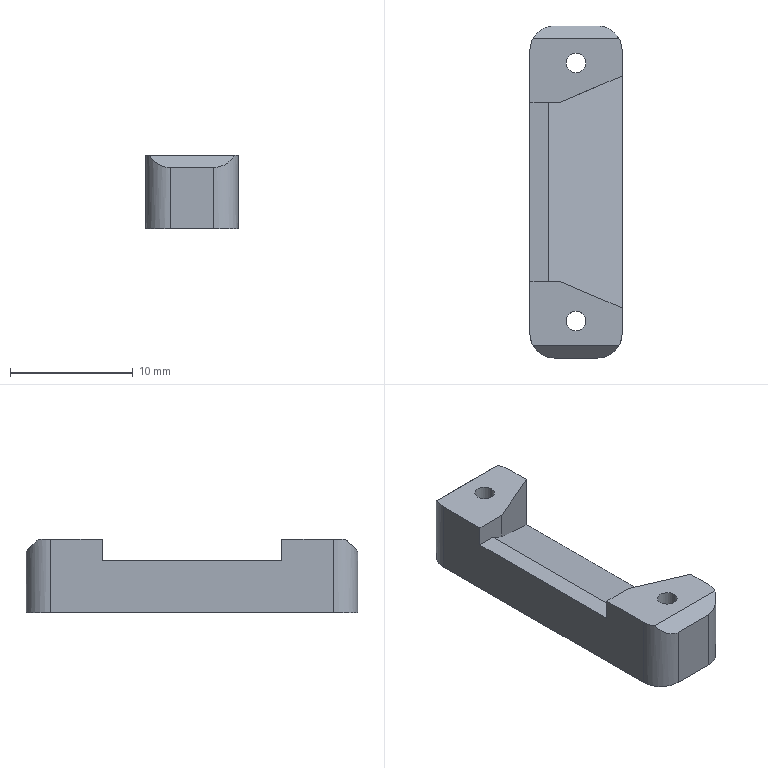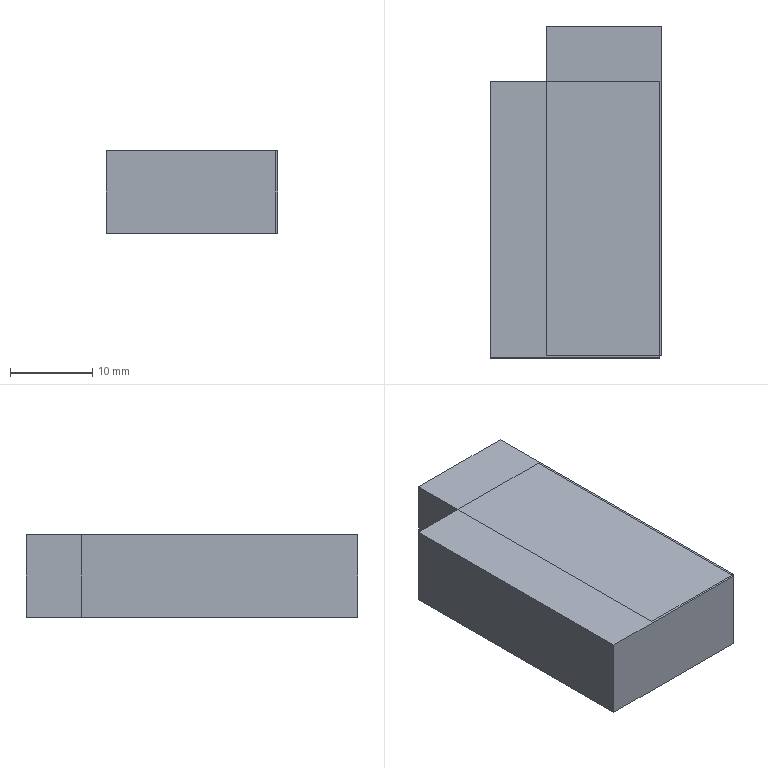CAM job | NX | 3+2 milling, drilling | part box 7.5 x 27 x 6 mm | stock box 20.75 x 40.25 x 10 mm
Tools:
number,name,description,diameter,corner_radius,flute_length,length,flutes
3,D3点钻,定心钻D4,3.0,0.0,43.0,75.0,2
1,D4-ROUGH,D4,4.0,0.0,12.0,50.0,2
2,D4-FINISH,D4,4.0,0.0,12.0,50.0,2
6,D4R0.3,Milling Tool-5 Parameters,4.0,0.3,50.0,75.0,2
4,D1.8钻头,Drilling Tool,1.8,0.0,35.0,50.0,2
5,M2丝攻,Drilling Tool,2.0,0.0,35.0,50.0,2
Operations:
program,operation,operation_type,tool,method,geometry_group,spindle_rpm,surface_speed,feed_per_tooth,feed_cut,feed_plunge,cut_length_mm,path_length_mm,cut_time_min,machine_time_min
XX-CNC1,FLOOR_FACING,VolumeBased25DMillingOperation,D4-ROUGH,METHOD,MCS_1,4500.0,100.0,0.1178,800.0,100.0,239.399,295.299,0.2992,0.3048
XX-CNC1,ADAPTIVE_MILLING,CavityMilling,D4-ROUGH,METHOD,W1,6500.0,100.0,0.1178,3000.0,100.0,1586.791,1927.42,0.5067,0.5407
XX-CNC1,FLOOR_FACING_COPY,VolumeBased25DMillingOperation,D4-FINISH,METHOD,MCS_1,4500.0,100.0,0.1178,800.0,100.0,239.399,295.399,0.2992,0.3048
XX-CNC1,PLANAR_MILL,PlanarMilling,D4-FINISH,METHOD,W1,5500.0,69.0,0.0727,800.0,100.0,177.562,247.562,0.222,0.229
XX-CNC1,FLOOR_FACING_1,VolumeBased25DMillingOperation,D4-FINISH,METHOD,W1,4500.0,100.0,0.1178,800.0,100.0,48.945,108.345,0.0612,0.0671
XX-CNC1,PLANAR_MILL_1,PlanarMilling,D4-FINISH,METHOD,W1,4500.0,100.0,0.1178,800.0,100.0,25.8,155.131,0.0323,0.0452
XX-CNC1,DRILLING,Operation,D3点钻,METHOD,W1,3000.0,0.0,0.0,200.0,0.0,8.0,100.213,0.04,0.0492
XX-CNC1,PLANAR_MILL_2,PlanarMilling,D3点钻,METHOD,W1,3500.0,100.0,0.1178,800.0,100.0,151.737,284.27,0.1897,0.2029
XX-CNC1,PLANAR_MILL_3,PlanarMilling,D3点钻,METHOD,W1,3500.0,100.0,0.1178,800.0,100.0,16.571,77.971,0.0207,0.0269
XX-CNC1,DRILLING_COPY,Operation,D1.8钻头,METHOD,W1,3000.0,0.0,0.0,150.0,0.0,22.0,128.213,0.1467,0.1573
XX-CNC1,DRILLING_COPY_COPY,Operation,M2丝攻,METHOD,W1,300.0,0.0,0.0,0.4,0.0,20.0,124.213,50.0,50.01
XX-CNC2,FLOOR_FACING_2,VolumeBased25DMillingOperation,D4-ROUGH,METHOD,MCS_2,4500.0,100.0,0.1178,800.0,100.0,69.563,125.363,0.087,0.0925
XX-CNC2,PLANAR_MILL_4,PlanarMilling,D4-ROUGH,METHOD,MCS_2,5000.0,100.0,0.1178,800.0,100.0,35.6,157.6,0.0445,0.0567
XX-CNC2,FLOOR_FACING_2_COPY,VolumeBased25DMillingOperation,D4-FINISH,METHOD,MCS_2,4500.0,100.0,0.1178,800.0,100.0,69.373,125.373,0.0867,0.0923
XX-CNC2,PLANAR_MILL_4_COPY,PlanarMilling,D4-FINISH,METHOD,MCS_2,5000.0,100.0,0.1178,800.0,100.0,36.326,158.856,0.0454,0.0577
XX-CNC2,ZLEVEL_PROFILE_STEEP,ZLevelMilling,D4R0.3,METHOD,MCS_2,4500.0,100.0,0.1178,1500.0,100.0,684.438,804.043,0.4563,0.4683
XX-CNC3,ADAPTIVE_MILLING_1,CavityMilling,D4-ROUGH,METHOD,W3,6500.0,81.0,0.2308,3000.0,100.0,1441.964,1495.764,0.4789,0.4843
XX-CNC3,FLOOR_FACING_3,VolumeBased25DMillingOperation,D4-FINISH,METHOD,MCS_3,5500.0,69.0,0.0727,800.0,100.0,105.854,161.854,0.1323,0.1379
XX-CNC3,PLANAR_MILL_5,PlanarMilling,D3点钻,METHOD,MCS_3,3500.0,100.0,0.1178,800.0,100.0,78.991,136.991,0.0987,0.1045
XX-CNC3,DRILLING_1,Operation,D3点钻,METHOD,MCS_3,3000.0,0.0,0.0,200.0,0.0,8.0,100.213,0.04,0.0492